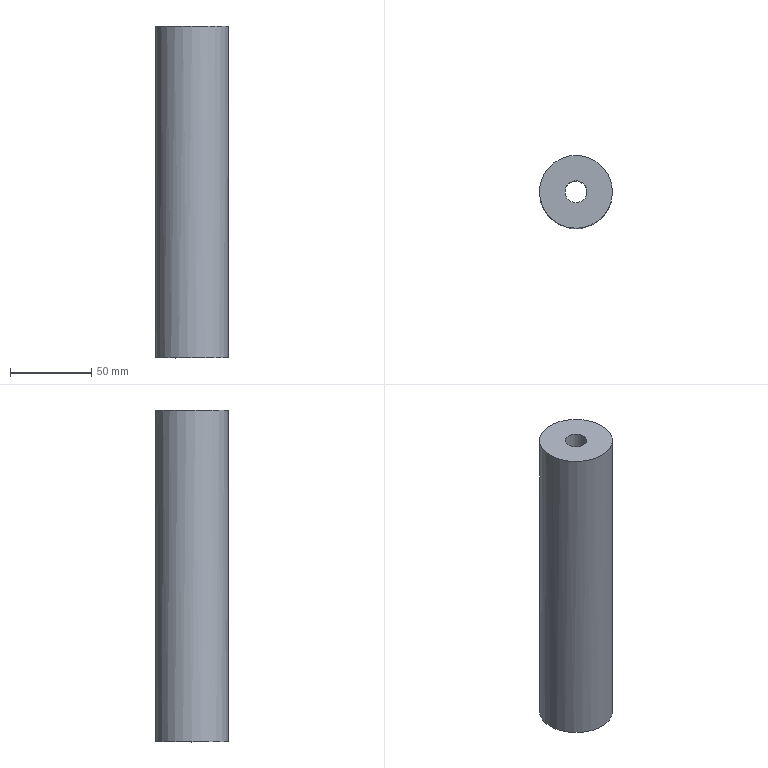Part | NX | features solid 2 | 1 solid | 6 faces | box 45 x 45 x 204.765 mm | volume 288664 mm3 | plane 3 | cylinder 3 | commonest cylinder face diameters 13.507 x1 20.008 x1 45 x1
STEP:
#1=CARTESIAN_POINT('',(1194.981,156.595,-23.635));
#2=VERTEX_POINT('',#1);
#3=CARTESIAN_POINT('',(1184.977,156.595,-23.635));
#4=DIRECTION('',(0.,0.,1.));
#5=DIRECTION('',(1.,0.,0.));
#6=AXIS2_PLACEMENT_3D('',#3,#4,#5);
#7=CIRCLE('',#6,10.004);
#8=EDGE_CURVE('',#2,#2,#7,.F.);
#9=ORIENTED_EDGE('',*,*,#8,.F.);
#10=EDGE_LOOP('',(#9));
#11=FACE_BOUND('',#10,.T.);
#12=CARTESIAN_POINT('',(1207.477,156.595,-23.635));
#13=VERTEX_POINT('',#12);
#14=CARTESIAN_POINT('',(1184.977,156.595,-23.635));
#15=DIRECTION('',(0.,0.,1.));
#16=DIRECTION('',(1.,0.,0.));
#17=AXIS2_PLACEMENT_3D('',#14,#15,#16);
#18=CIRCLE('',#17,22.5);
#19=EDGE_CURVE('',#13,#13,#18,.T.);
#20=ORIENTED_EDGE('',*,*,#19,.F.);
#21=EDGE_LOOP('',(#20));
#22=FACE_BOUND('',#21,.T.);
#23=CARTESIAN_POINT('',(1784.977,146.595,-23.635));
#24=DIRECTION('',(0.,0.,1.));
#25=DIRECTION('',(0.,1.,0.));
#26=AXIS2_PLACEMENT_3D('',#23,#24,#25);
#27=PLANE('',#26);
#28=ADVANCED_FACE('',(#11,#22),#27,.F.);
#29=ORIENTED_EDGE('',*,*,#19,.T.);
#30=EDGE_LOOP('',(#29));
#31=FACE_BOUND('',#30,.T.);
#32=CARTESIAN_POINT('',(1184.977,134.095,181.13));
#33=VERTEX_POINT('',#32);
#34=CARTESIAN_POINT('',(1184.977,156.595,181.13));
#35=DIRECTION('',(0.,0.,1.));
#36=DIRECTION('',(0.,-1.,0.));
#37=AXIS2_PLACEMENT_3D('',#34,#35,#36);
#38=CIRCLE('',#37,22.5);
#39=EDGE_CURVE('',#33,#33,#38,.T.);
#40=ORIENTED_EDGE('',*,*,#39,.F.);
#41=EDGE_LOOP('',(#40));
#42=FACE_BOUND('',#41,.T.);
#43=CARTESIAN_POINT('',(1184.977,156.595,-49.121));
#44=DIRECTION('',(0.,0.,-1.));
#45=DIRECTION('',(0.,1.,0.));
#46=AXIS2_PLACEMENT_3D('',#43,#44,#45);
#47=CYLINDRICAL_SURFACE('',#46,22.5);
#48=ADVANCED_FACE('',(#31,#42),#47,.T.);
#49=CARTESIAN_POINT('',(1184.977,149.842,181.13));
#50=VERTEX_POINT('',#49);
#51=CARTESIAN_POINT('',(1184.977,156.595,181.13));
#52=DIRECTION('',(0.,0.,1.));
#53=DIRECTION('',(0.,-1.,0.));
#54=AXIS2_PLACEMENT_3D('',#51,#52,#53);
#55=CIRCLE('',#54,6.753);
#56=EDGE_CURVE('',#50,#50,#55,.T.);
#57=ORIENTED_EDGE('',*,*,#56,.F.);
#58=EDGE_LOOP('',(#57));
#59=FACE_BOUND('',#58,.T.);
#60=ORIENTED_EDGE('',*,*,#39,.T.);
#61=EDGE_LOOP('',(#60));
#62=FACE_BOUND('',#61,.T.);
#63=CARTESIAN_POINT('',(1311.634,216.143,181.13));
#64=DIRECTION('',(0.,0.,1.));
#65=DIRECTION('',(0.,1.,0.));
#66=AXIS2_PLACEMENT_3D('',#63,#64,#65);
#67=PLANE('',#66);
#68=ADVANCED_FACE('',(#59,#62),#67,.T.);
#69=ORIENTED_EDGE('',*,*,#8,.T.);
#70=EDGE_LOOP('',(#69));
#71=FACE_BOUND('',#70,.T.);
#72=CARTESIAN_POINT('',(1174.973,156.595,21.129));
#73=VERTEX_POINT('',#72);
#74=CARTESIAN_POINT('',(1184.977,156.595,21.129));
#75=DIRECTION('',(0.,0.,1.));
#76=DIRECTION('',(-1.,0.,0.));
#77=AXIS2_PLACEMENT_3D('',#74,#75,#76);
#78=CIRCLE('',#77,10.004);
#79=EDGE_CURVE('',#73,#73,#78,.F.);
#80=ORIENTED_EDGE('',*,*,#79,.F.);
#81=EDGE_LOOP('',(#80));
#82=FACE_BOUND('',#81,.T.);
#83=CARTESIAN_POINT('',(1184.977,156.595,-23.871));
#84=DIRECTION('',(0.,0.,1.));
#85=DIRECTION('',(-1.,0.,0.));
#86=AXIS2_PLACEMENT_3D('',#83,#84,#85);
#87=CYLINDRICAL_SURFACE('',#86,10.004);
#88=ADVANCED_FACE('',(#71,#82),#87,.F.);
#89=CARTESIAN_POINT('',(1191.73,156.595,21.129));
#90=VERTEX_POINT('',#89);
#91=CARTESIAN_POINT('',(1184.977,156.595,21.129));
#92=DIRECTION('',(0.,0.,-1.));
#93=DIRECTION('',(1.,0.,0.));
#94=AXIS2_PLACEMENT_3D('',#91,#92,#93);
#95=CIRCLE('',#94,6.753);
#96=EDGE_CURVE('',#90,#90,#95,.T.);
#97=ORIENTED_EDGE('',*,*,#96,.T.);
#98=EDGE_LOOP('',(#97));
#99=FACE_BOUND('',#98,.T.);
#100=ORIENTED_EDGE('',*,*,#56,.T.);
#101=EDGE_LOOP('',(#100));
#102=FACE_BOUND('',#101,.T.);
#103=CARTESIAN_POINT('',(1184.977,156.595,-83.871));
#104=DIRECTION('',(0.,0.,1.));
#105=DIRECTION('',(-1.,0.,0.));
#106=AXIS2_PLACEMENT_3D('',#103,#104,#105);
#107=CYLINDRICAL_SURFACE('',#106,6.753);
#108=ADVANCED_FACE('',(#99,#102),#107,.F.);
#109=ORIENTED_EDGE('',*,*,#96,.F.);
#110=EDGE_LOOP('',(#109));
#111=FACE_BOUND('',#110,.T.);
#112=ORIENTED_EDGE('',*,*,#79,.T.);
#113=EDGE_LOOP('',(#112));
#114=FACE_BOUND('',#113,.T.);
#115=CARTESIAN_POINT('',(1184.977,156.595,21.129));
#116=DIRECTION('',(0.,0.,1.));
#117=DIRECTION('',(1.,0.,0.));
#118=AXIS2_PLACEMENT_3D('',#115,#116,#117);
#119=PLANE('',#118);
#120=ADVANCED_FACE('',(#111,#114),#119,.F.);
#121=CLOSED_SHELL('',(#28,#48,#68,#88,#108,#120));
#122=MANIFOLD_SOLID_BREP('',#121);
#123=(LENGTH_UNIT()NAMED_UNIT(*)SI_UNIT(.MILLI.,.METRE.));
#124=UNCERTAINTY_MEASURE_WITH_UNIT(LENGTH_MEASURE(0.00001),#123,'','');
#125=(NAMED_UNIT(*)PLANE_ANGLE_UNIT()SI_UNIT($,.RADIAN.));
#126=(NAMED_UNIT(*)SI_UNIT($,.STERADIAN.)SOLID_ANGLE_UNIT());
#127=(GEOMETRIC_REPRESENTATION_CONTEXT(3)GLOBAL_UNCERTAINTY_ASSIGNED_CONTEXT((#124))GLOBAL_UNIT_ASSIGNED_CONTEXT((#123,#125,#126))REPRESENTATION_CONTEXT('',''));
#128=ADVANCED_BREP_SHAPE_REPRESENTATION('',(#122),#127);